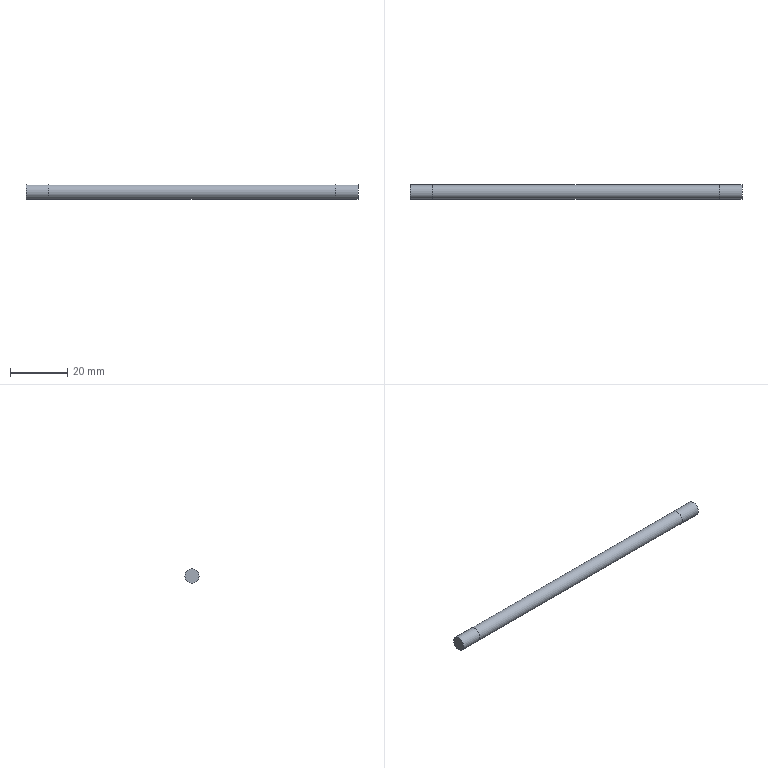Part | STEP file | 1-69.8 | 1 solid | 5 faces | box 116 x 5 x 5 mm | volume 2278 mm3 | cylinder 3 | plane 2 | commonest cylinder face diameters 5 x3
STEP:
#1=CARTESIAN_POINT('',(0.,0.,0.));
#2=DIRECTION('',(0.,0.,1.));
#3=DIRECTION('',(1.,0.,0.));
#4=AXIS2_PLACEMENT_3D('',#1,#2,#3);
#5=CARTESIAN_POINT('',(58.,2.5,0.));
#6=VERTEX_POINT('',#5);
#7=CARTESIAN_POINT('',(58.,0.,0.));
#8=DIRECTION('',(1.,0.,0.));
#9=DIRECTION('',(0.,1.,0.));
#10=AXIS2_PLACEMENT_3D('',#7,#8,#9);
#11=CIRCLE('',#10,2.5);
#12=CARTESIAN_POINT('',(58.,-0.6699,0.));
#13=DIRECTION('',(1.,0.,0.));
#14=DIRECTION('',(0.,1.,0.));
#15=AXIS2_PLACEMENT_3D('',#12,#13,#14);
#16=PLANE('',#15);
#17=CARTESIAN_POINT('',(0.6699,0.));
#18=DIRECTION('',(1.,0.));
#19=AXIS2_PLACEMENT_2D('',#17,#18);
#20=CIRCLE('',#19,2.5);
#21=(GEOMETRIC_REPRESENTATION_CONTEXT(2)PARAMETRIC_REPRESENTATION_CONTEXT()REPRESENTATION_CONTEXT('',''));
#22=DEFINITIONAL_REPRESENTATION('',(#20),#21);
#23=PCURVE('',#16,#22);
#24=CARTESIAN_POINT('',(58.,0.,0.));
#25=DIRECTION('',(-1.,0.,0.));
#26=DIRECTION('',(0.,1.,0.));
#27=AXIS2_PLACEMENT_3D('',#24,#25,#26);
#28=CYLINDRICAL_SURFACE('',#27,2.5);
#29=CARTESIAN_POINT('',(6.283,0.));
#30=DIRECTION('',(-1.,0.));
#31=VECTOR('',#30,1.);
#32=LINE('',#29,#31);
#33=(GEOMETRIC_REPRESENTATION_CONTEXT(2)PARAMETRIC_REPRESENTATION_CONTEXT()REPRESENTATION_CONTEXT('',''));
#34=DEFINITIONAL_REPRESENTATION('',(#32),#33);
#35=PCURVE('',#28,#34);
#36=SURFACE_CURVE('',#11,(#23,#35),.PCURVE_S1.);
#37=EDGE_CURVE('',#6,#6,#36,.T.);
#38=ORIENTED_EDGE('',*,*,#37,.T.);
#39=EDGE_LOOP('',(#38));
#40=FACE_BOUND('',#39,.T.);
#41=ADVANCED_FACE('',(#40),#16,.T.);
#42=CARTESIAN_POINT('',(-58.,2.5,0.));
#43=VERTEX_POINT('',#42);
#44=CARTESIAN_POINT('',(-58.,0.,0.));
#45=DIRECTION('',(1.,0.,0.));
#46=DIRECTION('',(0.,1.,0.));
#47=AXIS2_PLACEMENT_3D('',#44,#45,#46);
#48=CIRCLE('',#47,2.5);
#49=CARTESIAN_POINT('',(-58.,-0.6699,0.));
#50=DIRECTION('',(1.,0.,0.));
#51=DIRECTION('',(0.,1.,0.));
#52=AXIS2_PLACEMENT_3D('',#49,#50,#51);
#53=PLANE('',#52);
#54=CARTESIAN_POINT('',(0.6699,0.));
#55=DIRECTION('',(1.,0.));
#56=AXIS2_PLACEMENT_2D('',#54,#55);
#57=CIRCLE('',#56,2.5);
#58=(GEOMETRIC_REPRESENTATION_CONTEXT(2)PARAMETRIC_REPRESENTATION_CONTEXT()REPRESENTATION_CONTEXT('',''));
#59=DEFINITIONAL_REPRESENTATION('',(#57),#58);
#60=PCURVE('',#53,#59);
#61=CARTESIAN_POINT('',(-50.,0.,0.));
#62=DIRECTION('',(-1.,0.,0.));
#63=DIRECTION('',(0.,1.,0.));
#64=AXIS2_PLACEMENT_3D('',#61,#62,#63);
#65=CYLINDRICAL_SURFACE('',#64,2.5);
#66=CARTESIAN_POINT('',(6.283,8.));
#67=DIRECTION('',(-1.,0.));
#68=VECTOR('',#67,1.);
#69=LINE('',#66,#68);
#70=(GEOMETRIC_REPRESENTATION_CONTEXT(2)PARAMETRIC_REPRESENTATION_CONTEXT()REPRESENTATION_CONTEXT('',''));
#71=DEFINITIONAL_REPRESENTATION('',(#69),#70);
#72=PCURVE('',#65,#71);
#73=SURFACE_CURVE('',#48,(#60,#72),.PCURVE_S1.);
#74=EDGE_CURVE('',#43,#43,#73,.T.);
#75=ORIENTED_EDGE('',*,*,#74,.T.);
#76=EDGE_LOOP('',(#75));
#77=FACE_BOUND('',#76,.F.);
#78=ADVANCED_FACE('',(#77),#53,.F.);
#79=CARTESIAN_POINT('',(50.,2.5,0.));
#80=VERTEX_POINT('',#79);
#81=CARTESIAN_POINT('',(58.,2.5,0.));
#82=DIRECTION('',(-1.,0.,0.));
#83=VECTOR('',#82,1.);
#84=LINE('',#81,#83);
#85=CARTESIAN_POINT('',(6.283,0.));
#86=DIRECTION('',(0.,1.));
#87=VECTOR('',#86,1.);
#88=LINE('',#85,#87);
#89=(GEOMETRIC_REPRESENTATION_CONTEXT(2)PARAMETRIC_REPRESENTATION_CONTEXT()REPRESENTATION_CONTEXT('',''));
#90=DEFINITIONAL_REPRESENTATION('',(#88),#89);
#91=PCURVE('',#28,#90);
#92=CARTESIAN_POINT('',(0.,0.));
#93=DIRECTION('',(0.,1.));
#94=VECTOR('',#93,1.);
#95=LINE('',#92,#94);
#96=(GEOMETRIC_REPRESENTATION_CONTEXT(2)PARAMETRIC_REPRESENTATION_CONTEXT()REPRESENTATION_CONTEXT('',''));
#97=DEFINITIONAL_REPRESENTATION('',(#95),#96);
#98=PCURVE('',#28,#97);
#99=SEAM_CURVE('',#84,(#91,#98),.PCURVE_S1.);
#100=EDGE_CURVE('',#6,#80,#99,.T.);
#101=ORIENTED_EDGE('',*,*,#100,.T.);
#102=CARTESIAN_POINT('',(50.,0.,0.));
#103=DIRECTION('',(1.,0.,0.));
#104=DIRECTION('',(0.,1.,0.));
#105=AXIS2_PLACEMENT_3D('',#102,#103,#104);
#106=CIRCLE('',#105,2.5);
#107=CARTESIAN_POINT('',(6.283,8.));
#108=DIRECTION('',(-1.,0.));
#109=VECTOR('',#108,1.);
#110=LINE('',#107,#109);
#111=(GEOMETRIC_REPRESENTATION_CONTEXT(2)PARAMETRIC_REPRESENTATION_CONTEXT()REPRESENTATION_CONTEXT('',''));
#112=DEFINITIONAL_REPRESENTATION('',(#110),#111);
#113=PCURVE('',#28,#112);
#114=CARTESIAN_POINT('',(58.,0.,0.));
#115=DIRECTION('',(-1.,0.,0.));
#116=DIRECTION('',(0.,1.,0.));
#117=AXIS2_PLACEMENT_3D('',#114,#115,#116);
#118=CYLINDRICAL_SURFACE('',#117,2.5);
#119=CARTESIAN_POINT('',(6.283,8.));
#120=DIRECTION('',(-1.,0.));
#121=VECTOR('',#120,1.);
#122=LINE('',#119,#121);
#123=(GEOMETRIC_REPRESENTATION_CONTEXT(2)PARAMETRIC_REPRESENTATION_CONTEXT()REPRESENTATION_CONTEXT('',''));
#124=DEFINITIONAL_REPRESENTATION('',(#122),#123);
#125=PCURVE('',#118,#124);
#126=SURFACE_CURVE('',#106,(#113,#125),.PCURVE_S1.);
#127=EDGE_CURVE('',#80,#80,#126,.T.);
#128=ORIENTED_EDGE('',*,*,#127,.T.);
#129=ORIENTED_EDGE('',*,*,#100,.F.);
#130=ORIENTED_EDGE('',*,*,#37,.F.);
#131=EDGE_LOOP('',(#101,#128,#129,#130));
#132=FACE_BOUND('',#131,.T.);
#133=ADVANCED_FACE('',(#132),#28,.T.);
#134=CARTESIAN_POINT('',(-50.,2.5,0.));
#135=VERTEX_POINT('',#134);
#136=CARTESIAN_POINT('',(50.,2.5,0.));
#137=DIRECTION('',(-1.,0.,0.));
#138=VECTOR('',#137,1.);
#139=LINE('',#136,#138);
#140=CARTESIAN_POINT('',(6.283,8.));
#141=DIRECTION('',(0.,1.));
#142=VECTOR('',#141,1.);
#143=LINE('',#140,#142);
#144=(GEOMETRIC_REPRESENTATION_CONTEXT(2)PARAMETRIC_REPRESENTATION_CONTEXT()REPRESENTATION_CONTEXT('',''));
#145=DEFINITIONAL_REPRESENTATION('',(#143),#144);
#146=PCURVE('',#118,#145);
#147=CARTESIAN_POINT('',(0.,8.));
#148=DIRECTION('',(0.,1.));
#149=VECTOR('',#148,1.);
#150=LINE('',#147,#149);
#151=(GEOMETRIC_REPRESENTATION_CONTEXT(2)PARAMETRIC_REPRESENTATION_CONTEXT()REPRESENTATION_CONTEXT('',''));
#152=DEFINITIONAL_REPRESENTATION('',(#150),#151);
#153=PCURVE('',#118,#152);
#154=SEAM_CURVE('',#139,(#146,#153),.PCURVE_S1.);
#155=EDGE_CURVE('',#80,#135,#154,.T.);
#156=ORIENTED_EDGE('',*,*,#155,.T.);
#157=CARTESIAN_POINT('',(-50.,0.,0.));
#158=DIRECTION('',(1.,0.,0.));
#159=DIRECTION('',(0.,1.,0.));
#160=AXIS2_PLACEMENT_3D('',#157,#158,#159);
#161=CIRCLE('',#160,2.5);
#162=CARTESIAN_POINT('',(6.283,108.));
#163=DIRECTION('',(-1.,0.));
#164=VECTOR('',#163,1.);
#165=LINE('',#162,#164);
#166=(GEOMETRIC_REPRESENTATION_CONTEXT(2)PARAMETRIC_REPRESENTATION_CONTEXT()REPRESENTATION_CONTEXT('',''));
#167=DEFINITIONAL_REPRESENTATION('',(#165),#166);
#168=PCURVE('',#118,#167);
#169=CARTESIAN_POINT('',(6.283,0.));
#170=DIRECTION('',(-1.,0.));
#171=VECTOR('',#170,1.);
#172=LINE('',#169,#171);
#173=(GEOMETRIC_REPRESENTATION_CONTEXT(2)PARAMETRIC_REPRESENTATION_CONTEXT()REPRESENTATION_CONTEXT('',''));
#174=DEFINITIONAL_REPRESENTATION('',(#172),#173);
#175=PCURVE('',#65,#174);
#176=SURFACE_CURVE('',#161,(#168,#175),.PCURVE_S1.);
#177=EDGE_CURVE('',#135,#135,#176,.T.);
#178=ORIENTED_EDGE('',*,*,#177,.T.);
#179=ORIENTED_EDGE('',*,*,#155,.F.);
#180=ORIENTED_EDGE('',*,*,#127,.F.);
#181=EDGE_LOOP('',(#156,#178,#179,#180));
#182=FACE_BOUND('',#181,.T.);
#183=ADVANCED_FACE('',(#182),#118,.T.);
#184=CARTESIAN_POINT('',(-50.,2.5,0.));
#185=DIRECTION('',(-1.,0.,0.));
#186=VECTOR('',#185,1.);
#187=LINE('',#184,#186);
#188=CARTESIAN_POINT('',(0.,0.));
#189=DIRECTION('',(0.,1.));
#190=VECTOR('',#189,1.);
#191=LINE('',#188,#190);
#192=(GEOMETRIC_REPRESENTATION_CONTEXT(2)PARAMETRIC_REPRESENTATION_CONTEXT()REPRESENTATION_CONTEXT('',''));
#193=DEFINITIONAL_REPRESENTATION('',(#191),#192);
#194=PCURVE('',#65,#193);
#195=CARTESIAN_POINT('',(6.283,0.));
#196=DIRECTION('',(0.,1.));
#197=VECTOR('',#196,1.);
#198=LINE('',#195,#197);
#199=(GEOMETRIC_REPRESENTATION_CONTEXT(2)PARAMETRIC_REPRESENTATION_CONTEXT()REPRESENTATION_CONTEXT('',''));
#200=DEFINITIONAL_REPRESENTATION('',(#198),#199);
#201=PCURVE('',#65,#200);
#202=SEAM_CURVE('',#187,(#194,#201),.PCURVE_S1.);
#203=EDGE_CURVE('',#135,#43,#202,.T.);
#204=ORIENTED_EDGE('',*,*,#203,.F.);
#205=ORIENTED_EDGE('',*,*,#177,.F.);
#206=ORIENTED_EDGE('',*,*,#203,.T.);
#207=ORIENTED_EDGE('',*,*,#74,.T.);
#208=EDGE_LOOP('',(#204,#205,#206,#207));
#209=FACE_BOUND('',#208,.T.);
#210=ADVANCED_FACE('',(#209),#65,.T.);
#211=CLOSED_SHELL('',(#41,#78,#133,#183,#210));
#212=MANIFOLD_SOLID_BREP('',#211);
#213=(LENGTH_UNIT()NAMED_UNIT(*)SI_UNIT(.MILLI.,.METRE.));
#214=UNCERTAINTY_MEASURE_WITH_UNIT(LENGTH_MEASURE(0.0000001),#213,'','');
#215=(NAMED_UNIT(*)PLANE_ANGLE_UNIT()SI_UNIT($,.RADIAN.));
#216=(NAMED_UNIT(*)SI_UNIT($,.STERADIAN.)SOLID_ANGLE_UNIT());
#217=(GEOMETRIC_REPRESENTATION_CONTEXT(3)GLOBAL_UNCERTAINTY_ASSIGNED_CONTEXT((#214))GLOBAL_UNIT_ASSIGNED_CONTEXT((#213,#215,#216))REPRESENTATION_CONTEXT('',''));
#218=ADVANCED_BREP_SHAPE_REPRESENTATION('',(#4,#212),#217);